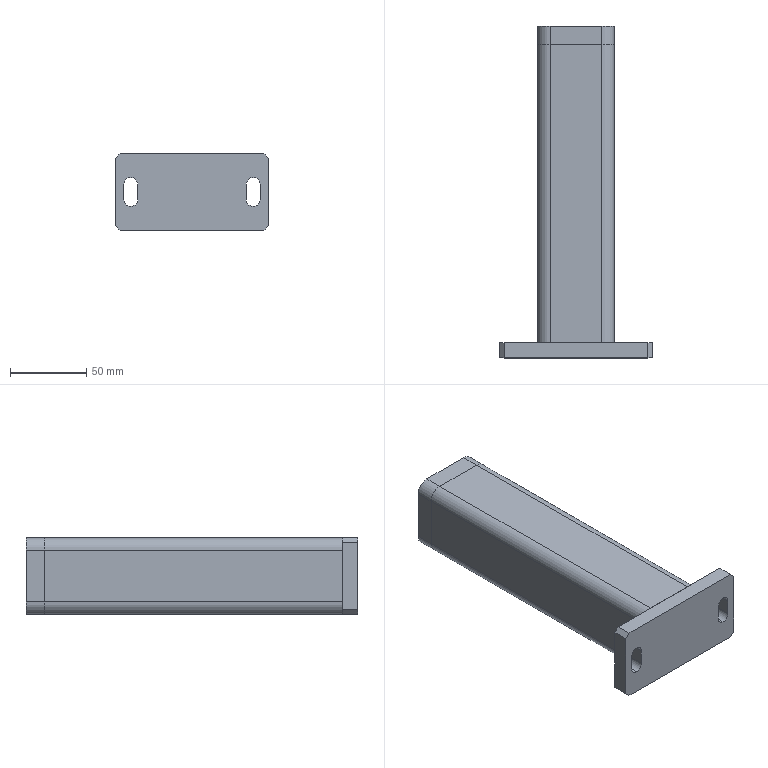Part | SolidWorks | features BaseBody 3 | 3 solids | 50 faces | box 100 x 217 x 50 mm | volume 210593 mm3 | plane 30 | cylinder 20 | commonest cylinder face diameters 16 x8 9 x6 8 x4 10.2 x2
STEP:
#1=CARTESIAN_POINT('',(21.,0.,-17.));
#2=VERTEX_POINT('',#1);
#3=CARTESIAN_POINT('',(17.,0.,-21.));
#4=VERTEX_POINT('',#3);
#5=CARTESIAN_POINT('',(17.,0.,-17.));
#6=DIRECTION('',(0.,1.,0.));
#7=DIRECTION('',(0.,0.,1.));
#8=AXIS2_PLACEMENT_3D('',#5,#6,#7);
#9=CIRCLE('',#8,4.);
#10=EDGE_CURVE('',#2,#4,#9,.T.);
#11=ORIENTED_EDGE('',*,*,#10,.T.);
#12=CARTESIAN_POINT('',(-17.,0.,-21.));
#13=VERTEX_POINT('',#12);
#14=CARTESIAN_POINT('',(-17.,0.,-21.));
#15=DIRECTION('',(-1.,0.,0.));
#16=VECTOR('',#15,1000.);
#17=LINE('',#14,#16);
#18=EDGE_CURVE('',#4,#13,#17,.T.);
#19=ORIENTED_EDGE('',*,*,#18,.T.);
#20=CARTESIAN_POINT('',(-21.,0.,-17.));
#21=VERTEX_POINT('',#20);
#22=CARTESIAN_POINT('',(-17.,0.,-17.));
#23=DIRECTION('',(0.,1.,0.));
#24=DIRECTION('',(0.,0.,1.));
#25=AXIS2_PLACEMENT_3D('',#22,#23,#24);
#26=CIRCLE('',#25,4.);
#27=EDGE_CURVE('',#13,#21,#26,.T.);
#28=ORIENTED_EDGE('',*,*,#27,.T.);
#29=CARTESIAN_POINT('',(-21.,0.,17.));
#30=VERTEX_POINT('',#29);
#31=CARTESIAN_POINT('',(-21.,0.,-17.));
#32=DIRECTION('',(0.,0.,1.));
#33=VECTOR('',#32,1000.);
#34=LINE('',#31,#33);
#35=EDGE_CURVE('',#21,#30,#34,.T.);
#36=ORIENTED_EDGE('',*,*,#35,.T.);
#37=CARTESIAN_POINT('',(-17.,0.,21.));
#38=VERTEX_POINT('',#37);
#39=CARTESIAN_POINT('',(-17.,0.,17.));
#40=DIRECTION('',(0.,1.,0.));
#41=DIRECTION('',(0.,0.,1.));
#42=AXIS2_PLACEMENT_3D('',#39,#40,#41);
#43=CIRCLE('',#42,4.);
#44=EDGE_CURVE('',#30,#38,#43,.T.);
#45=ORIENTED_EDGE('',*,*,#44,.T.);
#46=CARTESIAN_POINT('',(17.,0.,21.));
#47=VERTEX_POINT('',#46);
#48=CARTESIAN_POINT('',(17.,0.,21.));
#49=DIRECTION('',(1.,0.,0.));
#50=VECTOR('',#49,1000.);
#51=LINE('',#48,#50);
#52=EDGE_CURVE('',#38,#47,#51,.T.);
#53=ORIENTED_EDGE('',*,*,#52,.T.);
#54=CARTESIAN_POINT('',(21.,0.,17.));
#55=VERTEX_POINT('',#54);
#56=CARTESIAN_POINT('',(17.,0.,17.));
#57=DIRECTION('',(0.,1.,0.));
#58=DIRECTION('',(0.,0.,1.));
#59=AXIS2_PLACEMENT_3D('',#56,#57,#58);
#60=CIRCLE('',#59,4.);
#61=EDGE_CURVE('',#47,#55,#60,.T.);
#62=ORIENTED_EDGE('',*,*,#61,.T.);
#63=CARTESIAN_POINT('',(21.,0.,17.));
#64=DIRECTION('',(0.,0.,-1.));
#65=VECTOR('',#64,1000.);
#66=LINE('',#63,#65);
#67=EDGE_CURVE('',#55,#2,#66,.T.);
#68=ORIENTED_EDGE('',*,*,#67,.T.);
#69=EDGE_LOOP('',(#11,#19,#28,#36,#45,#53,#62,#68));
#70=FACE_BOUND('',#69,.T.);
#71=CARTESIAN_POINT('',(17.,0.,25.));
#72=VERTEX_POINT('',#71);
#73=CARTESIAN_POINT('',(25.,0.,17.));
#74=VERTEX_POINT('',#73);
#75=CARTESIAN_POINT('',(17.,0.,17.));
#76=DIRECTION('',(0.,1.,0.));
#77=DIRECTION('',(0.,0.,1.));
#78=AXIS2_PLACEMENT_3D('',#75,#76,#77);
#79=CIRCLE('',#78,8.);
#80=EDGE_CURVE('',#72,#74,#79,.T.);
#81=ORIENTED_EDGE('',*,*,#80,.F.);
#82=CARTESIAN_POINT('',(-17.,0.,25.));
#83=VERTEX_POINT('',#82);
#84=CARTESIAN_POINT('',(17.,0.,25.));
#85=DIRECTION('',(1.,0.,0.));
#86=VECTOR('',#85,1000.);
#87=LINE('',#84,#86);
#88=EDGE_CURVE('',#83,#72,#87,.T.);
#89=ORIENTED_EDGE('',*,*,#88,.F.);
#90=CARTESIAN_POINT('',(-25.,0.,17.));
#91=VERTEX_POINT('',#90);
#92=CARTESIAN_POINT('',(-17.,0.,17.));
#93=DIRECTION('',(0.,1.,0.));
#94=DIRECTION('',(0.,0.,1.));
#95=AXIS2_PLACEMENT_3D('',#92,#93,#94);
#96=CIRCLE('',#95,8.);
#97=EDGE_CURVE('',#91,#83,#96,.T.);
#98=ORIENTED_EDGE('',*,*,#97,.F.);
#99=CARTESIAN_POINT('',(-25.,0.,-17.));
#100=VERTEX_POINT('',#99);
#101=CARTESIAN_POINT('',(-25.,0.,-17.));
#102=DIRECTION('',(0.,0.,1.));
#103=VECTOR('',#102,1000.);
#104=LINE('',#101,#103);
#105=EDGE_CURVE('',#100,#91,#104,.T.);
#106=ORIENTED_EDGE('',*,*,#105,.F.);
#107=CARTESIAN_POINT('',(-17.,0.,-25.));
#108=VERTEX_POINT('',#107);
#109=CARTESIAN_POINT('',(-17.,0.,-17.));
#110=DIRECTION('',(0.,1.,0.));
#111=DIRECTION('',(0.,0.,1.));
#112=AXIS2_PLACEMENT_3D('',#109,#110,#111);
#113=CIRCLE('',#112,8.);
#114=EDGE_CURVE('',#108,#100,#113,.T.);
#115=ORIENTED_EDGE('',*,*,#114,.F.);
#116=CARTESIAN_POINT('',(17.,0.,-25.));
#117=VERTEX_POINT('',#116);
#118=CARTESIAN_POINT('',(-17.,0.,-25.));
#119=DIRECTION('',(-1.,0.,0.));
#120=VECTOR('',#119,1000.);
#121=LINE('',#118,#120);
#122=EDGE_CURVE('',#117,#108,#121,.T.);
#123=ORIENTED_EDGE('',*,*,#122,.F.);
#124=CARTESIAN_POINT('',(25.,0.,-17.));
#125=VERTEX_POINT('',#124);
#126=CARTESIAN_POINT('',(17.,0.,-17.));
#127=DIRECTION('',(0.,1.,0.));
#128=DIRECTION('',(0.,0.,1.));
#129=AXIS2_PLACEMENT_3D('',#126,#127,#128);
#130=CIRCLE('',#129,8.);
#131=EDGE_CURVE('',#125,#117,#130,.T.);
#132=ORIENTED_EDGE('',*,*,#131,.F.);
#133=CARTESIAN_POINT('',(25.,0.,17.));
#134=DIRECTION('',(0.,0.,-1.));
#135=VECTOR('',#134,1000.);
#136=LINE('',#133,#135);
#137=EDGE_CURVE('',#74,#125,#136,.T.);
#138=ORIENTED_EDGE('',*,*,#137,.F.);
#139=EDGE_LOOP('',(#81,#89,#98,#106,#115,#123,#132,#138));
#140=FACE_OUTER_BOUND('',#139,.T.);
#141=CARTESIAN_POINT('',(17.,0.,17.));
#142=DIRECTION('',(0.,1.,0.));
#143=DIRECTION('',(1.,0.,0.));
#144=AXIS2_PLACEMENT_3D('',#141,#142,#143);
#145=PLANE('',#144);
#146=ADVANCED_FACE('',(#70,#140),#145,.F.);
#147=CARTESIAN_POINT('',(21.,195.,-17.));
#148=VERTEX_POINT('',#147);
#149=CARTESIAN_POINT('',(17.,195.,-21.));
#150=VERTEX_POINT('',#149);
#151=CARTESIAN_POINT('',(17.,195.,-17.));
#152=DIRECTION('',(0.,1.,0.));
#153=DIRECTION('',(0.,0.,1.));
#154=AXIS2_PLACEMENT_3D('',#151,#152,#153);
#155=CIRCLE('',#154,4.);
#156=EDGE_CURVE('',#148,#150,#155,.T.);
#157=ORIENTED_EDGE('',*,*,#156,.F.);
#158=CARTESIAN_POINT('',(21.,195.,17.));
#159=VERTEX_POINT('',#158);
#160=CARTESIAN_POINT('',(21.,195.,17.));
#161=DIRECTION('',(0.,0.,-1.));
#162=VECTOR('',#161,1000.);
#163=LINE('',#160,#162);
#164=EDGE_CURVE('',#159,#148,#163,.T.);
#165=ORIENTED_EDGE('',*,*,#164,.F.);
#166=CARTESIAN_POINT('',(17.,195.,21.));
#167=VERTEX_POINT('',#166);
#168=CARTESIAN_POINT('',(17.,195.,17.));
#169=DIRECTION('',(0.,1.,0.));
#170=DIRECTION('',(0.,0.,1.));
#171=AXIS2_PLACEMENT_3D('',#168,#169,#170);
#172=CIRCLE('',#171,4.);
#173=EDGE_CURVE('',#167,#159,#172,.T.);
#174=ORIENTED_EDGE('',*,*,#173,.F.);
#175=CARTESIAN_POINT('',(-17.,195.,21.));
#176=VERTEX_POINT('',#175);
#177=CARTESIAN_POINT('',(17.,195.,21.));
#178=DIRECTION('',(1.,0.,0.));
#179=VECTOR('',#178,1000.);
#180=LINE('',#177,#179);
#181=EDGE_CURVE('',#176,#167,#180,.T.);
#182=ORIENTED_EDGE('',*,*,#181,.F.);
#183=CARTESIAN_POINT('',(-21.,195.,17.));
#184=VERTEX_POINT('',#183);
#185=CARTESIAN_POINT('',(-17.,195.,17.));
#186=DIRECTION('',(0.,1.,0.));
#187=DIRECTION('',(0.,0.,1.));
#188=AXIS2_PLACEMENT_3D('',#185,#186,#187);
#189=CIRCLE('',#188,4.);
#190=EDGE_CURVE('',#184,#176,#189,.T.);
#191=ORIENTED_EDGE('',*,*,#190,.F.);
#192=CARTESIAN_POINT('',(-21.,195.,-17.));
#193=VERTEX_POINT('',#192);
#194=CARTESIAN_POINT('',(-21.,195.,-17.));
#195=DIRECTION('',(0.,0.,1.));
#196=VECTOR('',#195,1000.);
#197=LINE('',#194,#196);
#198=EDGE_CURVE('',#193,#184,#197,.T.);
#199=ORIENTED_EDGE('',*,*,#198,.F.);
#200=CARTESIAN_POINT('',(-17.,195.,-21.));
#201=VERTEX_POINT('',#200);
#202=CARTESIAN_POINT('',(-17.,195.,-17.));
#203=DIRECTION('',(0.,1.,0.));
#204=DIRECTION('',(0.,0.,1.));
#205=AXIS2_PLACEMENT_3D('',#202,#203,#204);
#206=CIRCLE('',#205,4.);
#207=EDGE_CURVE('',#201,#193,#206,.T.);
#208=ORIENTED_EDGE('',*,*,#207,.F.);
#209=CARTESIAN_POINT('',(-17.,195.,-21.));
#210=DIRECTION('',(-1.,0.,0.));
#211=VECTOR('',#210,1000.);
#212=LINE('',#209,#211);
#213=EDGE_CURVE('',#150,#201,#212,.T.);
#214=ORIENTED_EDGE('',*,*,#213,.F.);
#215=EDGE_LOOP('',(#157,#165,#174,#182,#191,#199,#208,#214));
#216=FACE_BOUND('',#215,.T.);
#217=CARTESIAN_POINT('',(17.,195.,25.));
#218=VERTEX_POINT('',#217);
#219=CARTESIAN_POINT('',(25.,195.,17.));
#220=VERTEX_POINT('',#219);
#221=CARTESIAN_POINT('',(17.,195.,17.));
#222=DIRECTION('',(0.,1.,0.));
#223=DIRECTION('',(0.,0.,1.));
#224=AXIS2_PLACEMENT_3D('',#221,#222,#223);
#225=CIRCLE('',#224,8.);
#226=EDGE_CURVE('',#218,#220,#225,.T.);
#227=ORIENTED_EDGE('',*,*,#226,.T.);
#228=CARTESIAN_POINT('',(25.,195.,-17.));
#229=VERTEX_POINT('',#228);
#230=CARTESIAN_POINT('',(25.,195.,17.));
#231=DIRECTION('',(0.,0.,-1.));
#232=VECTOR('',#231,1000.);
#233=LINE('',#230,#232);
#234=EDGE_CURVE('',#220,#229,#233,.T.);
#235=ORIENTED_EDGE('',*,*,#234,.T.);
#236=CARTESIAN_POINT('',(17.,195.,-25.));
#237=VERTEX_POINT('',#236);
#238=CARTESIAN_POINT('',(17.,195.,-17.));
#239=DIRECTION('',(0.,1.,0.));
#240=DIRECTION('',(0.,0.,1.));
#241=AXIS2_PLACEMENT_3D('',#238,#239,#240);
#242=CIRCLE('',#241,8.);
#243=EDGE_CURVE('',#229,#237,#242,.T.);
#244=ORIENTED_EDGE('',*,*,#243,.T.);
#245=CARTESIAN_POINT('',(-17.,195.,-25.));
#246=VERTEX_POINT('',#245);
#247=CARTESIAN_POINT('',(-17.,195.,-25.));
#248=DIRECTION('',(-1.,0.,0.));
#249=VECTOR('',#248,1000.);
#250=LINE('',#247,#249);
#251=EDGE_CURVE('',#237,#246,#250,.T.);
#252=ORIENTED_EDGE('',*,*,#251,.T.);
#253=CARTESIAN_POINT('',(-25.,195.,-17.));
#254=VERTEX_POINT('',#253);
#255=CARTESIAN_POINT('',(-17.,195.,-17.));
#256=DIRECTION('',(0.,1.,0.));
#257=DIRECTION('',(0.,0.,1.));
#258=AXIS2_PLACEMENT_3D('',#255,#256,#257);
#259=CIRCLE('',#258,8.);
#260=EDGE_CURVE('',#246,#254,#259,.T.);
#261=ORIENTED_EDGE('',*,*,#260,.T.);
#262=CARTESIAN_POINT('',(-25.,195.,17.));
#263=VERTEX_POINT('',#262);
#264=CARTESIAN_POINT('',(-25.,195.,-17.));
#265=DIRECTION('',(0.,0.,1.));
#266=VECTOR('',#265,1000.);
#267=LINE('',#264,#266);
#268=EDGE_CURVE('',#254,#263,#267,.T.);
#269=ORIENTED_EDGE('',*,*,#268,.T.);
#270=CARTESIAN_POINT('',(-17.,195.,25.));
#271=VERTEX_POINT('',#270);
#272=CARTESIAN_POINT('',(-17.,195.,17.));
#273=DIRECTION('',(0.,1.,0.));
#274=DIRECTION('',(0.,0.,1.));
#275=AXIS2_PLACEMENT_3D('',#272,#273,#274);
#276=CIRCLE('',#275,8.);
#277=EDGE_CURVE('',#263,#271,#276,.T.);
#278=ORIENTED_EDGE('',*,*,#277,.T.);
#279=CARTESIAN_POINT('',(17.,195.,25.));
#280=DIRECTION('',(1.,0.,0.));
#281=VECTOR('',#280,1000.);
#282=LINE('',#279,#281);
#283=EDGE_CURVE('',#271,#218,#282,.T.);
#284=ORIENTED_EDGE('',*,*,#283,.T.);
#285=EDGE_LOOP('',(#227,#235,#244,#252,#261,#269,#278,#284));
#286=FACE_OUTER_BOUND('',#285,.T.);
#287=CARTESIAN_POINT('',(17.,195.,17.));
#288=DIRECTION('',(0.,1.,0.));
#289=DIRECTION('',(1.,0.,0.));
#290=AXIS2_PLACEMENT_3D('',#287,#288,#289);
#291=PLANE('',#290);
#292=ADVANCED_FACE('',(#216,#286),#291,.T.);
#293=ORIENTED_EDGE('',*,*,#88,.T.);
#294=CARTESIAN_POINT('',(17.,195.,25.));
#295=DIRECTION('',(0.,-1.,0.));
#296=VECTOR('',#295,1000.);
#297=LINE('',#294,#296);
#298=EDGE_CURVE('',#218,#72,#297,.T.);
#299=ORIENTED_EDGE('',*,*,#298,.F.);
#300=ORIENTED_EDGE('',*,*,#283,.F.);
#301=CARTESIAN_POINT('',(-17.,195.,25.));
#302=DIRECTION('',(0.,-1.,0.));
#303=VECTOR('',#302,1000.);
#304=LINE('',#301,#303);
#305=EDGE_CURVE('',#271,#83,#304,.T.);
#306=ORIENTED_EDGE('',*,*,#305,.T.);
#307=EDGE_LOOP('',(#293,#299,#300,#306));
#308=FACE_OUTER_BOUND('',#307,.T.);
#309=CARTESIAN_POINT('',(17.,195.,25.));
#310=DIRECTION('',(0.,0.,-1.));
#311=DIRECTION('',(0.,-1.,0.));
#312=AXIS2_PLACEMENT_3D('',#309,#310,#311);
#313=PLANE('',#312);
#314=ADVANCED_FACE('',(#308),#313,.F.);
#315=ORIENTED_EDGE('',*,*,#18,.F.);
#316=CARTESIAN_POINT('',(17.,195.,-21.));
#317=DIRECTION('',(0.,-1.,0.));
#318=VECTOR('',#317,1000.);
#319=LINE('',#316,#318);
#320=EDGE_CURVE('',#150,#4,#319,.T.);
#321=ORIENTED_EDGE('',*,*,#320,.F.);
#322=ORIENTED_EDGE('',*,*,#213,.T.);
#323=CARTESIAN_POINT('',(-17.,195.,-21.));
#324=DIRECTION('',(0.,-1.,0.));
#325=VECTOR('',#324,1000.);
#326=LINE('',#323,#325);
#327=EDGE_CURVE('',#201,#13,#326,.T.);
#328=ORIENTED_EDGE('',*,*,#327,.T.);
#329=EDGE_LOOP('',(#315,#321,#322,#328));
#330=FACE_OUTER_BOUND('',#329,.T.);
#331=CARTESIAN_POINT('',(-17.,195.,-21.));
#332=DIRECTION('',(0.,0.,1.));
#333=DIRECTION('',(1.,0.,0.));
#334=AXIS2_PLACEMENT_3D('',#331,#332,#333);
#335=PLANE('',#334);
#336=ADVANCED_FACE('',(#330),#335,.T.);
#337=ORIENTED_EDGE('',*,*,#27,.F.);
#338=ORIENTED_EDGE('',*,*,#327,.F.);
#339=ORIENTED_EDGE('',*,*,#207,.T.);
#340=CARTESIAN_POINT('',(-21.,195.,-17.));
#341=DIRECTION('',(0.,-1.,0.));
#342=VECTOR('',#341,1000.);
#343=LINE('',#340,#342);
#344=EDGE_CURVE('',#193,#21,#343,.T.);
#345=ORIENTED_EDGE('',*,*,#344,.T.);
#346=EDGE_LOOP('',(#337,#338,#339,#345));
#347=FACE_OUTER_BOUND('',#346,.T.);
#348=CARTESIAN_POINT('',(-17.,195.,-17.));
#349=DIRECTION('',(0.,-1.,0.));
#350=DIRECTION('',(0.,0.,-1.));
#351=AXIS2_PLACEMENT_3D('',#348,#349,#350);
#352=CYLINDRICAL_SURFACE('',#351,4.);
#353=ADVANCED_FACE('',(#347),#352,.F.);
#354=ORIENTED_EDGE('',*,*,#35,.F.);
#355=ORIENTED_EDGE('',*,*,#344,.F.);
#356=ORIENTED_EDGE('',*,*,#198,.T.);
#357=CARTESIAN_POINT('',(-21.,195.,17.));
#358=DIRECTION('',(0.,-1.,0.));
#359=VECTOR('',#358,1000.);
#360=LINE('',#357,#359);
#361=EDGE_CURVE('',#184,#30,#360,.T.);
#362=ORIENTED_EDGE('',*,*,#361,.T.);
#363=EDGE_LOOP('',(#354,#355,#356,#362));
#364=FACE_OUTER_BOUND('',#363,.T.);
#365=CARTESIAN_POINT('',(-21.,195.,-17.));
#366=DIRECTION('',(1.,0.,0.));
#367=DIRECTION('',(0.,1.,0.));
#368=AXIS2_PLACEMENT_3D('',#365,#366,#367);
#369=PLANE('',#368);
#370=ADVANCED_FACE('',(#364),#369,.T.);
#371=ORIENTED_EDGE('',*,*,#44,.F.);
#372=ORIENTED_EDGE('',*,*,#361,.F.);
#373=ORIENTED_EDGE('',*,*,#190,.T.);
#374=CARTESIAN_POINT('',(-17.,195.,21.));
#375=DIRECTION('',(0.,-1.,0.));
#376=VECTOR('',#375,1000.);
#377=LINE('',#374,#376);
#378=EDGE_CURVE('',#176,#38,#377,.T.);
#379=ORIENTED_EDGE('',*,*,#378,.T.);
#380=EDGE_LOOP('',(#371,#372,#373,#379));
#381=FACE_OUTER_BOUND('',#380,.T.);
#382=CARTESIAN_POINT('',(-17.,195.,17.));
#383=DIRECTION('',(0.,-1.,0.));
#384=DIRECTION('',(0.,0.,-1.));
#385=AXIS2_PLACEMENT_3D('',#382,#383,#384);
#386=CYLINDRICAL_SURFACE('',#385,4.);
#387=ADVANCED_FACE('',(#381),#386,.F.);
#388=ORIENTED_EDGE('',*,*,#52,.F.);
#389=ORIENTED_EDGE('',*,*,#378,.F.);
#390=ORIENTED_EDGE('',*,*,#181,.T.);
#391=CARTESIAN_POINT('',(17.,195.,21.));
#392=DIRECTION('',(0.,-1.,0.));
#393=VECTOR('',#392,1000.);
#394=LINE('',#391,#393);
#395=EDGE_CURVE('',#167,#47,#394,.T.);
#396=ORIENTED_EDGE('',*,*,#395,.T.);
#397=EDGE_LOOP('',(#388,#389,#390,#396));
#398=FACE_OUTER_BOUND('',#397,.T.);
#399=CARTESIAN_POINT('',(17.,195.,21.));
#400=DIRECTION('',(0.,0.,-1.));
#401=DIRECTION('',(0.,-1.,0.));
#402=AXIS2_PLACEMENT_3D('',#399,#400,#401);
#403=PLANE('',#402);
#404=ADVANCED_FACE('',(#398),#403,.T.);
#405=ORIENTED_EDGE('',*,*,#61,.F.);
#406=ORIENTED_EDGE('',*,*,#395,.F.);
#407=ORIENTED_EDGE('',*,*,#173,.T.);
#408=CARTESIAN_POINT('',(21.,195.,17.));
#409=DIRECTION('',(0.,-1.,0.));
#410=VECTOR('',#409,1000.);
#411=LINE('',#408,#410);
#412=EDGE_CURVE('',#159,#55,#411,.T.);
#413=ORIENTED_EDGE('',*,*,#412,.T.);
#414=EDGE_LOOP('',(#405,#406,#407,#413));
#415=FACE_OUTER_BOUND('',#414,.T.);
#416=CARTESIAN_POINT('',(17.,195.,17.));
#417=DIRECTION('',(0.,-1.,0.));
#418=DIRECTION('',(0.,0.,-1.));
#419=AXIS2_PLACEMENT_3D('',#416,#417,#418);
#420=CYLINDRICAL_SURFACE('',#419,4.);
#421=ADVANCED_FACE('',(#415),#420,.F.);
#422=ORIENTED_EDGE('',*,*,#67,.F.);
#423=ORIENTED_EDGE('',*,*,#412,.F.);
#424=ORIENTED_EDGE('',*,*,#164,.T.);
#425=CARTESIAN_POINT('',(21.,195.,-17.));
#426=DIRECTION('',(0.,-1.,0.));
#427=VECTOR('',#426,1000.);
#428=LINE('',#425,#427);
#429=EDGE_CURVE('',#148,#2,#428,.T.);
#430=ORIENTED_EDGE('',*,*,#429,.T.);
#431=EDGE_LOOP('',(#422,#423,#424,#430));
#432=FACE_OUTER_BOUND('',#431,.T.);
#433=CARTESIAN_POINT('',(21.,195.,17.));
#434=DIRECTION('',(-1.,0.,0.));
#435=DIRECTION('',(0.,0.,1.));
#436=AXIS2_PLACEMENT_3D('',#433,#434,#435);
#437=PLANE('',#436);
#438=ADVANCED_FACE('',(#432),#437,.T.);
#439=ORIENTED_EDGE('',*,*,#10,.F.);
#440=ORIENTED_EDGE('',*,*,#429,.F.);
#441=ORIENTED_EDGE('',*,*,#156,.T.);
#442=ORIENTED_EDGE('',*,*,#320,.T.);
#443=EDGE_LOOP('',(#439,#440,#441,#442));
#444=FACE_OUTER_BOUND('',#443,.T.);
#445=CARTESIAN_POINT('',(17.,195.,-17.));
#446=DIRECTION('',(0.,-1.,0.));
#447=DIRECTION('',(0.,0.,-1.));
#448=AXIS2_PLACEMENT_3D('',#445,#446,#447);
#449=CYLINDRICAL_SURFACE('',#448,4.);
#450=ADVANCED_FACE('',(#444),#449,.F.);
#451=ORIENTED_EDGE('',*,*,#97,.T.);
#452=ORIENTED_EDGE('',*,*,#305,.F.);
#453=ORIENTED_EDGE('',*,*,#277,.F.);
#454=CARTESIAN_POINT('',(-25.,195.,17.));
#455=DIRECTION('',(0.,-1.,0.));
#456=VECTOR('',#455,1000.);
#457=LINE('',#454,#456);
#458=EDGE_CURVE('',#263,#91,#457,.T.);
#459=ORIENTED_EDGE('',*,*,#458,.T.);
#460=EDGE_LOOP('',(#451,#452,#453,#459));
#461=FACE_OUTER_BOUND('',#460,.T.);
#462=CARTESIAN_POINT('',(-17.,195.,17.));
#463=DIRECTION('',(0.,-1.,0.));
#464=DIRECTION('',(0.,0.,-1.));
#465=AXIS2_PLACEMENT_3D('',#462,#463,#464);
#466=CYLINDRICAL_SURFACE('',#465,8.);
#467=ADVANCED_FACE('',(#461),#466,.T.);
#468=ORIENTED_EDGE('',*,*,#105,.T.);
#469=ORIENTED_EDGE('',*,*,#458,.F.);
#470=ORIENTED_EDGE('',*,*,#268,.F.);
#471=CARTESIAN_POINT('',(-25.,195.,-17.));
#472=DIRECTION('',(0.,-1.,0.));
#473=VECTOR('',#472,1000.);
#474=LINE('',#471,#473);
#475=EDGE_CURVE('',#254,#100,#474,.T.);
#476=ORIENTED_EDGE('',*,*,#475,.T.);
#477=EDGE_LOOP('',(#468,#469,#470,#476));
#478=FACE_OUTER_BOUND('',#477,.T.);
#479=CARTESIAN_POINT('',(-25.,195.,-17.));
#480=DIRECTION('',(1.,0.,0.));
#481=DIRECTION('',(0.,1.,0.));
#482=AXIS2_PLACEMENT_3D('',#479,#480,#481);
#483=PLANE('',#482);
#484=ADVANCED_FACE('',(#478),#483,.F.);
#485=ORIENTED_EDGE('',*,*,#114,.T.);
#486=ORIENTED_EDGE('',*,*,#475,.F.);
#487=ORIENTED_EDGE('',*,*,#260,.F.);
#488=CARTESIAN_POINT('',(-17.,195.,-25.));
#489=DIRECTION('',(0.,-1.,0.));
#490=VECTOR('',#489,1000.);
#491=LINE('',#488,#490);
#492=EDGE_CURVE('',#246,#108,#491,.T.);
#493=ORIENTED_EDGE('',*,*,#492,.T.);
#494=EDGE_LOOP('',(#485,#486,#487,#493));
#495=FACE_OUTER_BOUND('',#494,.T.);
#496=CARTESIAN_POINT('',(-17.,195.,-17.));
#497=DIRECTION('',(0.,-1.,0.));
#498=DIRECTION('',(0.,0.,-1.));
#499=AXIS2_PLACEMENT_3D('',#496,#497,#498);
#500=CYLINDRICAL_SURFACE('',#499,8.);
#501=ADVANCED_FACE('',(#495),#500,.T.);
#502=ORIENTED_EDGE('',*,*,#122,.T.);
#503=ORIENTED_EDGE('',*,*,#492,.F.);
#504=ORIENTED_EDGE('',*,*,#251,.F.);
#505=CARTESIAN_POINT('',(17.,195.,-25.));
#506=DIRECTION('',(0.,-1.,0.));
#507=VECTOR('',#506,1000.);
#508=LINE('',#505,#507);
#509=EDGE_CURVE('',#237,#117,#508,.T.);
#510=ORIENTED_EDGE('',*,*,#509,.T.);
#511=EDGE_LOOP('',(#502,#503,#504,#510));
#512=FACE_OUTER_BOUND('',#511,.T.);
#513=CARTESIAN_POINT('',(-17.,195.,-25.));
#514=DIRECTION('',(0.,0.,1.));
#515=DIRECTION('',(1.,0.,0.));
#516=AXIS2_PLACEMENT_3D('',#513,#514,#515);
#517=PLANE('',#516);
#518=ADVANCED_FACE('',(#512),#517,.F.);
#519=ORIENTED_EDGE('',*,*,#131,.T.);
#520=ORIENTED_EDGE('',*,*,#509,.F.);
#521=ORIENTED_EDGE('',*,*,#243,.F.);
#522=CARTESIAN_POINT('',(25.,195.,-17.));
#523=DIRECTION('',(0.,-1.,0.));
#524=VECTOR('',#523,1000.);
#525=LINE('',#522,#524);
#526=EDGE_CURVE('',#229,#125,#525,.T.);
#527=ORIENTED_EDGE('',*,*,#526,.T.);
#528=EDGE_LOOP('',(#519,#520,#521,#527));
#529=FACE_OUTER_BOUND('',#528,.T.);
#530=CARTESIAN_POINT('',(17.,195.,-17.));
#531=DIRECTION('',(0.,-1.,0.));
#532=DIRECTION('',(0.,0.,-1.));
#533=AXIS2_PLACEMENT_3D('',#530,#531,#532);
#534=CYLINDRICAL_SURFACE('',#533,8.);
#535=ADVANCED_FACE('',(#529),#534,.T.);
#536=ORIENTED_EDGE('',*,*,#137,.T.);
#537=ORIENTED_EDGE('',*,*,#526,.F.);
#538=ORIENTED_EDGE('',*,*,#234,.F.);
#539=CARTESIAN_POINT('',(25.,195.,17.));
#540=DIRECTION('',(0.,-1.,0.));
#541=VECTOR('',#540,1000.);
#542=LINE('',#539,#541);
#543=EDGE_CURVE('',#220,#74,#542,.T.);
#544=ORIENTED_EDGE('',*,*,#543,.T.);
#545=EDGE_LOOP('',(#536,#537,#538,#544));
#546=FACE_OUTER_BOUND('',#545,.T.);
#547=CARTESIAN_POINT('',(25.,195.,17.));
#548=DIRECTION('',(-1.,0.,0.));
#549=DIRECTION('',(0.,0.,1.));
#550=AXIS2_PLACEMENT_3D('',#547,#548,#549);
#551=PLANE('',#550);
#552=ADVANCED_FACE('',(#546),#551,.F.);
#553=ORIENTED_EDGE('',*,*,#80,.T.);
#554=ORIENTED_EDGE('',*,*,#543,.F.);
#555=ORIENTED_EDGE('',*,*,#226,.F.);
#556=ORIENTED_EDGE('',*,*,#298,.T.);
#557=EDGE_LOOP('',(#553,#554,#555,#556));
#558=FACE_OUTER_BOUND('',#557,.T.);
#559=CARTESIAN_POINT('',(17.,195.,17.));
#560=DIRECTION('',(0.,-1.,0.));
#561=DIRECTION('',(0.,0.,-1.));
#562=AXIS2_PLACEMENT_3D('',#559,#560,#561);
#563=CYLINDRICAL_SURFACE('',#562,8.);
#564=ADVANCED_FACE('',(#558),#563,.T.);
#565=CLOSED_SHELL('',(#146,#292,#314,#336,#353,#370,#387,#404,#421,#438,#450,#467,#484,#501,#518,#535,#552,#564));
#566=MANIFOLD_SOLID_BREP('',#565);
#567=CARTESIAN_POINT('',(0.,195.,-5.1));
#568=VERTEX_POINT('',#567);
#569=CARTESIAN_POINT('',(0.,207.,-5.1));
#570=VERTEX_POINT('',#569);
#571=CARTESIAN_POINT('',(0.,207.,-5.1));
#572=DIRECTION('',(0.,1.,0.));
#573=VECTOR('',#572,1000.);
#574=LINE('',#571,#573);
#575=EDGE_CURVE('',#568,#570,#574,.T.);
#576=ORIENTED_EDGE('',*,*,#575,.F.);
#577=CARTESIAN_POINT('',(0.,195.,5.1));
#578=VERTEX_POINT('',#577);
#579=CARTESIAN_POINT('',(0.,195.,0.));
#580=DIRECTION('',(0.,1.,0.));
#581=DIRECTION('',(0.,0.,1.));
#582=AXIS2_PLACEMENT_3D('',#579,#580,#581);
#583=CIRCLE('',#582,5.1);
#584=EDGE_CURVE('',#578,#568,#583,.T.);
#585=ORIENTED_EDGE('',*,*,#584,.F.);
#586=CARTESIAN_POINT('',(0.,207.,5.1));
#587=VERTEX_POINT('',#586);
#588=CARTESIAN_POINT('',(0.,207.,5.1));
#589=DIRECTION('',(0.,1.,0.));
#590=VECTOR('',#589,1000.);
#591=LINE('',#588,#590);
#592=EDGE_CURVE('',#578,#587,#591,.T.);
#593=ORIENTED_EDGE('',*,*,#592,.T.);
#594=CARTESIAN_POINT('',(0.,207.,0.));
#595=DIRECTION('',(0.,1.,0.));
#596=DIRECTION('',(0.,0.,1.));
#597=AXIS2_PLACEMENT_3D('',#594,#595,#596);
#598=CIRCLE('',#597,5.1);
#599=EDGE_CURVE('',#587,#570,#598,.T.);
#600=ORIENTED_EDGE('',*,*,#599,.T.);
#601=EDGE_LOOP('',(#576,#585,#593,#600));
#602=FACE_OUTER_BOUND('',#601,.T.);
#603=CARTESIAN_POINT('',(0.,207.,0.));
#604=DIRECTION('',(0.,1.,0.));
#605=DIRECTION('',(0.,0.,1.));
#606=AXIS2_PLACEMENT_3D('',#603,#604,#605);
#607=CYLINDRICAL_SURFACE('',#606,5.1);
#608=ADVANCED_FACE('',(#602),#607,.F.);
#609=ORIENTED_EDGE('',*,*,#584,.T.);
#610=CARTESIAN_POINT('',(0.,195.,0.));
#611=DIRECTION('',(0.,1.,0.));
#612=DIRECTION('',(0.,0.,1.));
#613=AXIS2_PLACEMENT_3D('',#610,#611,#612);
#614=CIRCLE('',#613,5.1);
#615=EDGE_CURVE('',#568,#578,#614,.T.);
#616=ORIENTED_EDGE('',*,*,#615,.T.);
#617=EDGE_LOOP('',(#609,#616));
#618=FACE_BOUND('',#617,.T.);
#619=CARTESIAN_POINT('',(17.,195.,25.));
#620=VERTEX_POINT('',#619);
#621=CARTESIAN_POINT('',(25.,195.,17.));
#622=VERTEX_POINT('',#621);
#623=CARTESIAN_POINT('',(17.,195.,17.));
#624=DIRECTION('',(0.,1.,0.));
#625=DIRECTION('',(0.,0.,1.));
#626=AXIS2_PLACEMENT_3D('',#623,#624,#625);
#627=CIRCLE('',#626,8.);
#628=EDGE_CURVE('',#620,#622,#627,.T.);
#629=ORIENTED_EDGE('',*,*,#628,.F.);
#630=CARTESIAN_POINT('',(-17.,195.,25.));
#631=VERTEX_POINT('',#630);
#632=CARTESIAN_POINT('',(-17.,195.,25.));
#633=DIRECTION('',(1.,0.,0.));
#634=VECTOR('',#633,1000.);
#635=LINE('',#632,#634);
#636=EDGE_CURVE('',#631,#620,#635,.T.);
#637=ORIENTED_EDGE('',*,*,#636,.F.);
#638=CARTESIAN_POINT('',(-25.,195.,17.));
#639=VERTEX_POINT('',#638);
#640=CARTESIAN_POINT('',(-17.,195.,17.));
#641=DIRECTION('',(0.,1.,0.));
#642=DIRECTION('',(0.,0.,1.));
#643=AXIS2_PLACEMENT_3D('',#640,#641,#642);
#644=CIRCLE('',#643,8.);
#645=EDGE_CURVE('',#639,#631,#644,.T.);
#646=ORIENTED_EDGE('',*,*,#645,.F.);
#647=CARTESIAN_POINT('',(-25.,195.,-17.));
#648=VERTEX_POINT('',#647);
#649=CARTESIAN_POINT('',(-25.,195.,-17.));
#650=DIRECTION('',(0.,0.,1.));
#651=VECTOR('',#650,1000.);
#652=LINE('',#649,#651);
#653=EDGE_CURVE('',#648,#639,#652,.T.);
#654=ORIENTED_EDGE('',*,*,#653,.F.);
#655=CARTESIAN_POINT('',(-17.,195.,-25.));
#656=VERTEX_POINT('',#655);
#657=CARTESIAN_POINT('',(-17.,195.,-17.));
#658=DIRECTION('',(0.,1.,0.));
#659=DIRECTION('',(0.,0.,1.));
#660=AXIS2_PLACEMENT_3D('',#657,#658,#659);
#661=CIRCLE('',#660,8.);
#662=EDGE_CURVE('',#656,#648,#661,.T.);
#663=ORIENTED_EDGE('',*,*,#662,.F.);
#664=CARTESIAN_POINT('',(17.,195.,-25.));
#665=VERTEX_POINT('',#664);
#666=CARTESIAN_POINT('',(17.,195.,-25.));
#667=DIRECTION('',(-1.,0.,0.));
#668=VECTOR('',#667,1000.);
#669=LINE('',#666,#668);
#670=EDGE_CURVE('',#665,#656,#669,.T.);
#671=ORIENTED_EDGE('',*,*,#670,.F.);
#672=CARTESIAN_POINT('',(25.,195.,-17.));
#673=VERTEX_POINT('',#672);
#674=CARTESIAN_POINT('',(17.,195.,-17.));
#675=DIRECTION('',(0.,1.,0.));
#676=DIRECTION('',(0.,0.,1.));
#677=AXIS2_PLACEMENT_3D('',#674,#675,#676);
#678=CIRCLE('',#677,8.);
#679=EDGE_CURVE('',#673,#665,#678,.T.);
#680=ORIENTED_EDGE('',*,*,#679,.F.);
#681=CARTESIAN_POINT('',(25.,195.,17.));
#682=DIRECTION('',(0.,0.,-1.));
#683=VECTOR('',#682,1000.);
#684=LINE('',#681,#683);
#685=EDGE_CURVE('',#622,#673,#684,.T.);
#686=ORIENTED_EDGE('',*,*,#685,.F.);
#687=EDGE_LOOP('',(#629,#637,#646,#654,#663,#671,#680,#686));
#688=FACE_OUTER_BOUND('',#687,.T.);
#689=CARTESIAN_POINT('',(17.,195.,17.));
#690=DIRECTION('',(0.,1.,0.));
#691=DIRECTION('',(1.,0.,0.));
#692=AXIS2_PLACEMENT_3D('',#689,#690,#691);
#693=PLANE('',#692);
#694=ADVANCED_FACE('',(#618,#688),#693,.F.);
#695=ORIENTED_EDGE('',*,*,#599,.F.);
#696=CARTESIAN_POINT('',(0.,207.,0.));
#697=DIRECTION('',(0.,1.,0.));
#698=DIRECTION('',(0.,0.,1.));
#699=AXIS2_PLACEMENT_3D('',#696,#697,#698);
#700=CIRCLE('',#699,5.1);
#701=EDGE_CURVE('',#570,#587,#700,.T.);
#702=ORIENTED_EDGE('',*,*,#701,.F.);
#703=EDGE_LOOP('',(#695,#702));
#704=FACE_BOUND('',#703,.T.);
#705=CARTESIAN_POINT('',(17.,207.,25.));
#706=VERTEX_POINT('',#705);
#707=CARTESIAN_POINT('',(25.,207.,17.));
#708=VERTEX_POINT('',#707);
#709=CARTESIAN_POINT('',(17.,207.,17.));
#710=DIRECTION('',(0.,1.,0.));
#711=DIRECTION('',(0.,0.,1.));
#712=AXIS2_PLACEMENT_3D('',#709,#710,#711);
#713=CIRCLE('',#712,8.);
#714=EDGE_CURVE('',#706,#708,#713,.T.);
#715=ORIENTED_EDGE('',*,*,#714,.T.);
#716=CARTESIAN_POINT('',(25.,207.,-17.));
#717=VERTEX_POINT('',#716);
#718=CARTESIAN_POINT('',(25.,207.,17.));
#719=DIRECTION('',(0.,0.,-1.));
#720=VECTOR('',#719,1000.);
#721=LINE('',#718,#720);
#722=EDGE_CURVE('',#708,#717,#721,.T.);
#723=ORIENTED_EDGE('',*,*,#722,.T.);
#724=CARTESIAN_POINT('',(17.,207.,-25.));
#725=VERTEX_POINT('',#724);
#726=CARTESIAN_POINT('',(17.,207.,-17.));
#727=DIRECTION('',(0.,1.,0.));
#728=DIRECTION('',(0.,0.,1.));
#729=AXIS2_PLACEMENT_3D('',#726,#727,#728);
#730=CIRCLE('',#729,8.);
#731=EDGE_CURVE('',#717,#725,#730,.T.);
#732=ORIENTED_EDGE('',*,*,#731,.T.);
#733=CARTESIAN_POINT('',(-17.,207.,-25.));
#734=VERTEX_POINT('',#733);
#735=CARTESIAN_POINT('',(17.,207.,-25.));
#736=DIRECTION('',(-1.,0.,0.));
#737=VECTOR('',#736,1000.);
#738=LINE('',#735,#737);
#739=EDGE_CURVE('',#725,#734,#738,.T.);
#740=ORIENTED_EDGE('',*,*,#739,.T.);
#741=CARTESIAN_POINT('',(-25.,207.,-17.));
#742=VERTEX_POINT('',#741);
#743=CARTESIAN_POINT('',(-17.,207.,-17.));
#744=DIRECTION('',(0.,1.,0.));
#745=DIRECTION('',(0.,0.,1.));
#746=AXIS2_PLACEMENT_3D('',#743,#744,#745);
#747=CIRCLE('',#746,8.);
#748=EDGE_CURVE('',#734,#742,#747,.T.);
#749=ORIENTED_EDGE('',*,*,#748,.T.);
#750=CARTESIAN_POINT('',(-25.,207.,17.));
#751=VERTEX_POINT('',#750);
#752=CARTESIAN_POINT('',(-25.,207.,-17.));
#753=DIRECTION('',(0.,0.,1.));
#754=VECTOR('',#753,1000.);
#755=LINE('',#752,#754);
#756=EDGE_CURVE('',#742,#751,#755,.T.);
#757=ORIENTED_EDGE('',*,*,#756,.T.);
#758=CARTESIAN_POINT('',(-17.,207.,25.));
#759=VERTEX_POINT('',#758);
#760=CARTESIAN_POINT('',(-17.,207.,17.));
#761=DIRECTION('',(0.,1.,0.));
#762=DIRECTION('',(0.,0.,1.));
#763=AXIS2_PLACEMENT_3D('',#760,#761,#762);
#764=CIRCLE('',#763,8.);
#765=EDGE_CURVE('',#751,#759,#764,.T.);
#766=ORIENTED_EDGE('',*,*,#765,.T.);
#767=CARTESIAN_POINT('',(-17.,207.,25.));
#768=DIRECTION('',(1.,0.,0.));
#769=VECTOR('',#768,1000.);
#770=LINE('',#767,#769);
#771=EDGE_CURVE('',#759,#706,#770,.T.);
#772=ORIENTED_EDGE('',*,*,#771,.T.);
#773=EDGE_LOOP('',(#715,#723,#732,#740,#749,#757,#766,#772));
#774=FACE_OUTER_BOUND('',#773,.T.);
#775=CARTESIAN_POINT('',(17.,207.,17.));
#776=DIRECTION('',(0.,1.,0.));
#777=DIRECTION('',(1.,0.,0.));
#778=AXIS2_PLACEMENT_3D('',#775,#776,#777);
#779=PLANE('',#778);
#780=ADVANCED_FACE('',(#704,#774),#779,.T.);
#781=ORIENTED_EDGE('',*,*,#636,.T.);
#782=CARTESIAN_POINT('',(17.,207.,25.));
#783=DIRECTION('',(0.,-1.,0.));
#784=VECTOR('',#783,1000.);
#785=LINE('',#782,#784);
#786=EDGE_CURVE('',#706,#620,#785,.T.);
#787=ORIENTED_EDGE('',*,*,#786,.F.);
#788=ORIENTED_EDGE('',*,*,#771,.F.);
#789=CARTESIAN_POINT('',(-17.,207.,25.));
#790=DIRECTION('',(0.,-1.,0.));
#791=VECTOR('',#790,1000.);
#792=LINE('',#789,#791);
#793=EDGE_CURVE('',#759,#631,#792,.T.);
#794=ORIENTED_EDGE('',*,*,#793,.T.);
#795=EDGE_LOOP('',(#781,#787,#788,#794));
#796=FACE_OUTER_BOUND('',#795,.T.);
#797=CARTESIAN_POINT('',(-17.,207.,25.));
#798=DIRECTION('',(0.,0.,-1.));
#799=DIRECTION('',(0.,-1.,0.));
#800=AXIS2_PLACEMENT_3D('',#797,#798,#799);
#801=PLANE('',#800);
#802=ADVANCED_FACE('',(#796),#801,.F.);
#803=ORIENTED_EDGE('',*,*,#645,.T.);
#804=ORIENTED_EDGE('',*,*,#793,.F.);
#805=ORIENTED_EDGE('',*,*,#765,.F.);
#806=CARTESIAN_POINT('',(-25.,207.,17.));
#807=DIRECTION('',(0.,-1.,0.));
#808=VECTOR('',#807,1000.);
#809=LINE('',#806,#808);
#810=EDGE_CURVE('',#751,#639,#809,.T.);
#811=ORIENTED_EDGE('',*,*,#810,.T.);
#812=EDGE_LOOP('',(#803,#804,#805,#811));
#813=FACE_OUTER_BOUND('',#812,.T.);
#814=CARTESIAN_POINT('',(-17.,207.,17.));
#815=DIRECTION('',(0.,-1.,0.));
#816=DIRECTION('',(0.,0.,-1.));
#817=AXIS2_PLACEMENT_3D('',#814,#815,#816);
#818=CYLINDRICAL_SURFACE('',#817,8.);
#819=ADVANCED_FACE('',(#813),#818,.T.);
#820=ORIENTED_EDGE('',*,*,#653,.T.);
#821=ORIENTED_EDGE('',*,*,#810,.F.);
#822=ORIENTED_EDGE('',*,*,#756,.F.);
#823=CARTESIAN_POINT('',(-25.,207.,-17.));
#824=DIRECTION('',(0.,-1.,0.));
#825=VECTOR('',#824,1000.);
#826=LINE('',#823,#825);
#827=EDGE_CURVE('',#742,#648,#826,.T.);
#828=ORIENTED_EDGE('',*,*,#827,.T.);
#829=EDGE_LOOP('',(#820,#821,#822,#828));
#830=FACE_OUTER_BOUND('',#829,.T.);
#831=CARTESIAN_POINT('',(-25.,207.,-17.));
#832=DIRECTION('',(1.,0.,0.));
#833=DIRECTION('',(0.,0.,1.));
#834=AXIS2_PLACEMENT_3D('',#831,#832,#833);
#835=PLANE('',#834);
#836=ADVANCED_FACE('',(#830),#835,.F.);
#837=ORIENTED_EDGE('',*,*,#662,.T.);
#838=ORIENTED_EDGE('',*,*,#827,.F.);
#839=ORIENTED_EDGE('',*,*,#748,.F.);
#840=CARTESIAN_POINT('',(-17.,207.,-25.));
#841=DIRECTION('',(0.,-1.,0.));
#842=VECTOR('',#841,1000.);
#843=LINE('',#840,#842);
#844=EDGE_CURVE('',#734,#656,#843,.T.);
#845=ORIENTED_EDGE('',*,*,#844,.T.);
#846=EDGE_LOOP('',(#837,#838,#839,#845));
#847=FACE_OUTER_BOUND('',#846,.T.);
#848=CARTESIAN_POINT('',(-17.,207.,-17.));
#849=DIRECTION('',(0.,-1.,0.));
#850=DIRECTION('',(0.,0.,-1.));
#851=AXIS2_PLACEMENT_3D('',#848,#849,#850);
#852=CYLINDRICAL_SURFACE('',#851,8.);
#853=ADVANCED_FACE('',(#847),#852,.T.);
#854=ORIENTED_EDGE('',*,*,#670,.T.);
#855=ORIENTED_EDGE('',*,*,#844,.F.);
#856=ORIENTED_EDGE('',*,*,#739,.F.);
#857=CARTESIAN_POINT('',(17.,207.,-25.));
#858=DIRECTION('',(0.,-1.,0.));
#859=VECTOR('',#858,1000.);
#860=LINE('',#857,#859);
#861=EDGE_CURVE('',#725,#665,#860,.T.);
#862=ORIENTED_EDGE('',*,*,#861,.T.);
#863=EDGE_LOOP('',(#854,#855,#856,#862));
#864=FACE_OUTER_BOUND('',#863,.T.);
#865=CARTESIAN_POINT('',(17.,207.,-25.));
#866=DIRECTION('',(0.,0.,1.));
#867=DIRECTION('',(1.,0.,0.));
#868=AXIS2_PLACEMENT_3D('',#865,#866,#867);
#869=PLANE('',#868);
#870=ADVANCED_FACE('',(#864),#869,.F.);
#871=ORIENTED_EDGE('',*,*,#679,.T.);
#872=ORIENTED_EDGE('',*,*,#861,.F.);
#873=ORIENTED_EDGE('',*,*,#731,.F.);
#874=CARTESIAN_POINT('',(25.,207.,-17.));
#875=DIRECTION('',(0.,-1.,0.));
#876=VECTOR('',#875,1000.);
#877=LINE('',#874,#876);
#878=EDGE_CURVE('',#717,#673,#877,.T.);
#879=ORIENTED_EDGE('',*,*,#878,.T.);
#880=EDGE_LOOP('',(#871,#872,#873,#879));
#881=FACE_OUTER_BOUND('',#880,.T.);
#882=CARTESIAN_POINT('',(17.,207.,-17.));
#883=DIRECTION('',(0.,-1.,0.));
#884=DIRECTION('',(0.,0.,-1.));
#885=AXIS2_PLACEMENT_3D('',#882,#883,#884);
#886=CYLINDRICAL_SURFACE('',#885,8.);
#887=ADVANCED_FACE('',(#881),#886,.T.);
#888=ORIENTED_EDGE('',*,*,#685,.T.);
#889=ORIENTED_EDGE('',*,*,#878,.F.);
#890=ORIENTED_EDGE('',*,*,#722,.F.);
#891=CARTESIAN_POINT('',(25.,207.,17.));
#892=DIRECTION('',(0.,-1.,0.));
#893=VECTOR('',#892,1000.);
#894=LINE('',#891,#893);
#895=EDGE_CURVE('',#708,#622,#894,.T.);
#896=ORIENTED_EDGE('',*,*,#895,.T.);
#897=EDGE_LOOP('',(#888,#889,#890,#896));
#898=FACE_OUTER_BOUND('',#897,.T.);
#899=CARTESIAN_POINT('',(25.,207.,17.));
#900=DIRECTION('',(-1.,0.,0.));
#901=DIRECTION('',(0.,0.,1.));
#902=AXIS2_PLACEMENT_3D('',#899,#900,#901);
#903=PLANE('',#902);
#904=ADVANCED_FACE('',(#898),#903,.F.);
#905=ORIENTED_EDGE('',*,*,#628,.T.);
#906=ORIENTED_EDGE('',*,*,#895,.F.);
#907=ORIENTED_EDGE('',*,*,#714,.F.);
#908=ORIENTED_EDGE('',*,*,#786,.T.);
#909=EDGE_LOOP('',(#905,#906,#907,#908));
#910=FACE_OUTER_BOUND('',#909,.T.);
#911=CARTESIAN_POINT('',(17.,207.,17.));
#912=DIRECTION('',(0.,-1.,0.));
#913=DIRECTION('',(0.,0.,-1.));
#914=AXIS2_PLACEMENT_3D('',#911,#912,#913);
#915=CYLINDRICAL_SURFACE('',#914,8.);
#916=ADVANCED_FACE('',(#910),#915,.T.);
#917=ORIENTED_EDGE('',*,*,#615,.F.);
#918=ORIENTED_EDGE('',*,*,#575,.T.);
#919=ORIENTED_EDGE('',*,*,#701,.T.);
#920=ORIENTED_EDGE('',*,*,#592,.F.);
#921=EDGE_LOOP('',(#917,#918,#919,#920));
#922=FACE_OUTER_BOUND('',#921,.T.);
#923=CARTESIAN_POINT('',(0.,207.,0.));
#924=DIRECTION('',(0.,1.,0.));
#925=DIRECTION('',(0.,0.,1.));
#926=AXIS2_PLACEMENT_3D('',#923,#924,#925);
#927=CYLINDRICAL_SURFACE('',#926,5.1);
#928=ADVANCED_FACE('',(#922),#927,.F.);
#929=CLOSED_SHELL('',(#608,#694,#780,#802,#819,#836,#853,#870,#887,#904,#916,#928));
#930=MANIFOLD_SOLID_BREP('',#929);
#931=CARTESIAN_POINT('',(-35.5,-10.,5.));
#932=VERTEX_POINT('',#931);
#933=CARTESIAN_POINT('',(-35.5,0.,5.));
#934=VERTEX_POINT('',#933);
#935=CARTESIAN_POINT('',(-35.5,207.,5.));
#936=DIRECTION('',(0.,1.,0.));
#937=VECTOR('',#936,1000.);
#938=LINE('',#935,#937);
#939=EDGE_CURVE('',#932,#934,#938,.T.);
#940=ORIENTED_EDGE('',*,*,#939,.F.);
#941=CARTESIAN_POINT('',(-44.5,-10.,5.));
#942=VERTEX_POINT('',#941);
#943=CARTESIAN_POINT('',(-40.,-10.,5.));
#944=DIRECTION('',(0.,-1.,0.));
#945=DIRECTION('',(0.,0.,-1.));
#946=AXIS2_PLACEMENT_3D('',#943,#944,#945);
#947=CIRCLE('',#946,4.5);
#948=EDGE_CURVE('',#932,#942,#947,.T.);
#949=ORIENTED_EDGE('',*,*,#948,.T.);
#950=CARTESIAN_POINT('',(-44.5,0.,5.));
#951=VERTEX_POINT('',#950);
#952=CARTESIAN_POINT('',(-44.5,-10.,5.));
#953=DIRECTION('',(0.,-1.,0.));
#954=VECTOR('',#953,1000.);
#955=LINE('',#952,#954);
#956=EDGE_CURVE('',#951,#942,#955,.T.);
#957=ORIENTED_EDGE('',*,*,#956,.F.);
#958=CARTESIAN_POINT('',(-40.,0.,5.));
#959=DIRECTION('',(0.,-1.,0.));
#960=DIRECTION('',(0.,0.,-1.));
#961=AXIS2_PLACEMENT_3D('',#958,#959,#960);
#962=CIRCLE('',#961,4.5);
#963=EDGE_CURVE('',#934,#951,#962,.T.);
#964=ORIENTED_EDGE('',*,*,#963,.F.);
#965=EDGE_LOOP('',(#940,#949,#957,#964));
#966=FACE_OUTER_BOUND('',#965,.T.);
#967=CARTESIAN_POINT('',(-40.,-10.,5.));
#968=DIRECTION('',(0.,-1.,0.));
#969=DIRECTION('',(0.,0.,-1.));
#970=AXIS2_PLACEMENT_3D('',#967,#968,#969);
#971=CYLINDRICAL_SURFACE('',#970,4.5);
#972=ADVANCED_FACE('',(#966),#971,.F.);
#973=ORIENTED_EDGE('',*,*,#956,.T.);
#974=CARTESIAN_POINT('',(-44.5,-10.,-5.));
#975=VERTEX_POINT('',#974);
#976=CARTESIAN_POINT('',(-44.5,-10.,-5.));
#977=DIRECTION('',(0.,0.,1.));
#978=VECTOR('',#977,1000.);
#979=LINE('',#976,#978);
#980=EDGE_CURVE('',#975,#942,#979,.T.);
#981=ORIENTED_EDGE('',*,*,#980,.F.);
#982=CARTESIAN_POINT('',(-44.5,0.,-5.));
#983=VERTEX_POINT('',#982);
#984=CARTESIAN_POINT('',(-44.5,-10.,-5.));
#985=DIRECTION('',(0.,1.,0.));
#986=VECTOR('',#985,1000.);
#987=LINE('',#984,#986);
#988=EDGE_CURVE('',#975,#983,#987,.T.);
#989=ORIENTED_EDGE('',*,*,#988,.T.);
#990=CARTESIAN_POINT('',(-44.5,0.,0.));
#991=DIRECTION('',(0.,0.,-1.));
#992=VECTOR('',#991,1000.);
#993=LINE('',#990,#992);
#994=EDGE_CURVE('',#951,#983,#993,.T.);
#995=ORIENTED_EDGE('',*,*,#994,.F.);
#996=EDGE_LOOP('',(#973,#981,#989,#995));
#997=FACE_OUTER_BOUND('',#996,.T.);
#998=CARTESIAN_POINT('',(-44.5,-10.,-5.));
#999=DIRECTION('',(-1.,0.,0.));
#1000=DIRECTION('',(0.,0.,1.));
#1001=AXIS2_PLACEMENT_3D('',#998,#999,#1000);
#1002=PLANE('',#1001);
#1003=ADVANCED_FACE('',(#997),#1002,.F.);
#1004=CARTESIAN_POINT('',(-40.,0.,-9.5));
#1005=VERTEX_POINT('',#1004);
#1006=CARTESIAN_POINT('',(-40.,-10.,-9.5));
#1007=VERTEX_POINT('',#1006);
#1008=CARTESIAN_POINT('',(-40.,-10.,-9.5));
#1009=DIRECTION('',(0.,-1.,0.));
#1010=VECTOR('',#1009,1000.);
#1011=LINE('',#1008,#1010);
#1012=EDGE_CURVE('',#1005,#1007,#1011,.T.);
#1013=ORIENTED_EDGE('',*,*,#1012,.F.);
#1014=CARTESIAN_POINT('',(-40.,0.,-5.));
#1015=DIRECTION('',(0.,-1.,0.));
#1016=DIRECTION('',(0.,0.,-1.));
#1017=AXIS2_PLACEMENT_3D('',#1014,#1015,#1016);
#1018=CIRCLE('',#1017,4.5);
#1019=EDGE_CURVE('',#983,#1005,#1018,.T.);
#1020=ORIENTED_EDGE('',*,*,#1019,.F.);
#1021=ORIENTED_EDGE('',*,*,#988,.F.);
#1022=CARTESIAN_POINT('',(-40.,-10.,-5.));
#1023=DIRECTION('',(0.,-1.,0.));
#1024=DIRECTION('',(0.,0.,-1.));
#1025=AXIS2_PLACEMENT_3D('',#1022,#1023,#1024);
#1026=CIRCLE('',#1025,4.5);
#1027=EDGE_CURVE('',#975,#1007,#1026,.T.);
#1028=ORIENTED_EDGE('',*,*,#1027,.T.);
#1029=EDGE_LOOP('',(#1013,#1020,#1021,#1028));
#1030=FACE_OUTER_BOUND('',#1029,.T.);
#1031=CARTESIAN_POINT('',(-40.,-10.,-5.));
#1032=DIRECTION('',(0.,-1.,0.));
#1033=DIRECTION('',(0.,0.,-1.));
#1034=AXIS2_PLACEMENT_3D('',#1031,#1032,#1033);
#1035=CYLINDRICAL_SURFACE('',#1034,4.5);
#1036=ADVANCED_FACE('',(#1030),#1035,.F.);
#1037=CARTESIAN_POINT('',(-35.5,-10.,-5.));
#1038=VERTEX_POINT('',#1037);
#1039=CARTESIAN_POINT('',(-35.5,0.,-5.));
#1040=VERTEX_POINT('',#1039);
#1041=CARTESIAN_POINT('',(-35.5,207.,-5.));
#1042=DIRECTION('',(0.,1.,0.));
#1043=VECTOR('',#1042,1000.);
#1044=LINE('',#1041,#1043);
#1045=EDGE_CURVE('',#1038,#1040,#1044,.T.);
#1046=ORIENTED_EDGE('',*,*,#1045,.F.);
#1047=CARTESIAN_POINT('',(-35.5,-10.,-5.));
#1048=DIRECTION('',(0.,0.,1.));
#1049=VECTOR('',#1048,1000.);
#1050=LINE('',#1047,#1049);
#1051=EDGE_CURVE('',#1038,#932,#1050,.T.);
#1052=ORIENTED_EDGE('',*,*,#1051,.T.);
#1053=ORIENTED_EDGE('',*,*,#939,.T.);
#1054=CARTESIAN_POINT('',(-35.5,0.,0.));
#1055=DIRECTION('',(0.,0.,1.));
#1056=VECTOR('',#1055,1000.);
#1057=LINE('',#1054,#1056);
#1058=EDGE_CURVE('',#1040,#934,#1057,.T.);
#1059=ORIENTED_EDGE('',*,*,#1058,.F.);
#1060=EDGE_LOOP('',(#1046,#1052,#1053,#1059));
#1061=FACE_OUTER_BOUND('',#1060,.T.);
#1062=CARTESIAN_POINT('',(-35.5,207.,-5.));
#1063=DIRECTION('',(1.,0.,0.));
#1064=DIRECTION('',(0.,1.,0.));
#1065=AXIS2_PLACEMENT_3D('',#1062,#1063,#1064);
#1066=PLANE('',#1065);
#1067=ADVANCED_FACE('',(#1061),#1066,.F.);
#1068=CARTESIAN_POINT('',(44.5,-10.,5.));
#1069=VERTEX_POINT('',#1068);
#1070=CARTESIAN_POINT('',(44.5,0.,5.));
#1071=VERTEX_POINT('',#1070);
#1072=CARTESIAN_POINT('',(44.5,207.,5.));
#1073=DIRECTION('',(0.,1.,0.));
#1074=VECTOR('',#1073,1000.);
#1075=LINE('',#1072,#1074);
#1076=EDGE_CURVE('',#1069,#1071,#1075,.T.);
#1077=ORIENTED_EDGE('',*,*,#1076,.F.);
#1078=CARTESIAN_POINT('',(35.5,-10.,5.));
#1079=VERTEX_POINT('',#1078);
#1080=CARTESIAN_POINT('',(40.,-10.,5.));
#1081=DIRECTION('',(0.,-1.,0.));
#1082=DIRECTION('',(0.,0.,-1.));
#1083=AXIS2_PLACEMENT_3D('',#1080,#1081,#1082);
#1084=CIRCLE('',#1083,4.5);
#1085=EDGE_CURVE('',#1069,#1079,#1084,.T.);
#1086=ORIENTED_EDGE('',*,*,#1085,.T.);
#1087=CARTESIAN_POINT('',(35.5,0.,5.));
#1088=VERTEX_POINT('',#1087);
#1089=CARTESIAN_POINT('',(35.5,-10.,5.));
#1090=DIRECTION('',(0.,-1.,0.));
#1091=VECTOR('',#1090,1000.);
#1092=LINE('',#1089,#1091);
#1093=EDGE_CURVE('',#1088,#1079,#1092,.T.);
#1094=ORIENTED_EDGE('',*,*,#1093,.F.);
#1095=CARTESIAN_POINT('',(40.,0.,5.));
#1096=DIRECTION('',(0.,-1.,0.));
#1097=DIRECTION('',(0.,0.,-1.));
#1098=AXIS2_PLACEMENT_3D('',#1095,#1096,#1097);
#1099=CIRCLE('',#1098,4.5);
#1100=EDGE_CURVE('',#1071,#1088,#1099,.T.);
#1101=ORIENTED_EDGE('',*,*,#1100,.F.);
#1102=EDGE_LOOP('',(#1077,#1086,#1094,#1101));
#1103=FACE_OUTER_BOUND('',#1102,.T.);
#1104=CARTESIAN_POINT('',(40.,-10.,5.));
#1105=DIRECTION('',(0.,-1.,0.));
#1106=DIRECTION('',(0.,0.,-1.));
#1107=AXIS2_PLACEMENT_3D('',#1104,#1105,#1106);
#1108=CYLINDRICAL_SURFACE('',#1107,4.5);
#1109=ADVANCED_FACE('',(#1103),#1108,.F.);
#1110=CARTESIAN_POINT('',(44.5,-10.,-5.));
#1111=VERTEX_POINT('',#1110);
#1112=CARTESIAN_POINT('',(44.5,0.,-5.));
#1113=VERTEX_POINT('',#1112);
#1114=CARTESIAN_POINT('',(44.5,207.,-5.));
#1115=DIRECTION('',(0.,1.,0.));
#1116=VECTOR('',#1115,1000.);
#1117=LINE('',#1114,#1116);
#1118=EDGE_CURVE('',#1111,#1113,#1117,.T.);
#1119=ORIENTED_EDGE('',*,*,#1118,.F.);
#1120=CARTESIAN_POINT('',(44.5,-10.,-5.));
#1121=DIRECTION('',(0.,0.,1.));
#1122=VECTOR('',#1121,1000.);
#1123=LINE('',#1120,#1122);
#1124=EDGE_CURVE('',#1111,#1069,#1123,.T.);
#1125=ORIENTED_EDGE('',*,*,#1124,.T.);
#1126=ORIENTED_EDGE('',*,*,#1076,.T.);
#1127=CARTESIAN_POINT('',(44.5,0.,0.));
#1128=DIRECTION('',(0.,0.,1.));
#1129=VECTOR('',#1128,1000.);
#1130=LINE('',#1127,#1129);
#1131=EDGE_CURVE('',#1113,#1071,#1130,.T.);
#1132=ORIENTED_EDGE('',*,*,#1131,.F.);
#1133=EDGE_LOOP('',(#1119,#1125,#1126,#1132));
#1134=FACE_OUTER_BOUND('',#1133,.T.);
#1135=CARTESIAN_POINT('',(44.5,207.,-5.));
#1136=DIRECTION('',(1.,0.,0.));
#1137=DIRECTION('',(0.,1.,0.));
#1138=AXIS2_PLACEMENT_3D('',#1135,#1136,#1137);
#1139=PLANE('',#1138);
#1140=ADVANCED_FACE('',(#1134),#1139,.F.);
#1141=CARTESIAN_POINT('',(40.,0.,-9.5));
#1142=VERTEX_POINT('',#1141);
#1143=CARTESIAN_POINT('',(40.,-10.,-9.5));
#1144=VERTEX_POINT('',#1143);
#1145=CARTESIAN_POINT('',(40.,-10.,-9.5));
#1146=DIRECTION('',(0.,-1.,0.));
#1147=VECTOR('',#1146,1000.);
#1148=LINE('',#1145,#1147);
#1149=EDGE_CURVE('',#1142,#1144,#1148,.T.);
#1150=ORIENTED_EDGE('',*,*,#1149,.F.);
#1151=CARTESIAN_POINT('',(35.5,0.,-5.));
#1152=VERTEX_POINT('',#1151);
#1153=CARTESIAN_POINT('',(40.,0.,-5.));
#1154=DIRECTION('',(0.,-1.,0.));
#1155=DIRECTION('',(0.,0.,-1.));
#1156=AXIS2_PLACEMENT_3D('',#1153,#1154,#1155);
#1157=CIRCLE('',#1156,4.5);
#1158=EDGE_CURVE('',#1152,#1142,#1157,.T.);
#1159=ORIENTED_EDGE('',*,*,#1158,.F.);
#1160=CARTESIAN_POINT('',(35.5,-10.,-5.));
#1161=VERTEX_POINT('',#1160);
#1162=CARTESIAN_POINT('',(35.5,-10.,-5.));
#1163=DIRECTION('',(0.,1.,0.));
#1164=VECTOR('',#1163,1000.);
#1165=LINE('',#1162,#1164);
#1166=EDGE_CURVE('',#1161,#1152,#1165,.T.);
#1167=ORIENTED_EDGE('',*,*,#1166,.F.);
#1168=CARTESIAN_POINT('',(40.,-10.,-5.));
#1169=DIRECTION('',(0.,-1.,0.));
#1170=DIRECTION('',(0.,0.,-1.));
#1171=AXIS2_PLACEMENT_3D('',#1168,#1169,#1170);
#1172=CIRCLE('',#1171,4.5);
#1173=EDGE_CURVE('',#1161,#1144,#1172,.T.);
#1174=ORIENTED_EDGE('',*,*,#1173,.T.);
#1175=EDGE_LOOP('',(#1150,#1159,#1167,#1174));
#1176=FACE_OUTER_BOUND('',#1175,.T.);
#1177=CARTESIAN_POINT('',(40.,-10.,-5.));
#1178=DIRECTION('',(0.,-1.,0.));
#1179=DIRECTION('',(0.,0.,-1.));
#1180=AXIS2_PLACEMENT_3D('',#1177,#1178,#1179);
#1181=CYLINDRICAL_SURFACE('',#1180,4.5);
#1182=ADVANCED_FACE('',(#1176),#1181,.F.);
#1183=ORIENTED_EDGE('',*,*,#1093,.T.);
#1184=CARTESIAN_POINT('',(35.5,-10.,-5.));
#1185=DIRECTION('',(0.,0.,1.));
#1186=VECTOR('',#1185,1000.);
#1187=LINE('',#1184,#1186);
#1188=EDGE_CURVE('',#1161,#1079,#1187,.T.);
#1189=ORIENTED_EDGE('',*,*,#1188,.F.);
#1190=ORIENTED_EDGE('',*,*,#1166,.T.);
#1191=CARTESIAN_POINT('',(35.5,0.,0.));
#1192=DIRECTION('',(0.,0.,-1.));
#1193=VECTOR('',#1192,1000.);
#1194=LINE('',#1191,#1193);
#1195=EDGE_CURVE('',#1088,#1152,#1194,.T.);
#1196=ORIENTED_EDGE('',*,*,#1195,.F.);
#1197=EDGE_LOOP('',(#1183,#1189,#1190,#1196));
#1198=FACE_OUTER_BOUND('',#1197,.T.);
#1199=CARTESIAN_POINT('',(35.5,-10.,-5.));
#1200=DIRECTION('',(-1.,0.,0.));
#1201=DIRECTION('',(0.,0.,1.));
#1202=AXIS2_PLACEMENT_3D('',#1199,#1200,#1201);
#1203=PLANE('',#1202);
#1204=ADVANCED_FACE('',(#1198),#1203,.F.);
#1205=ORIENTED_EDGE('',*,*,#1131,.T.);
#1206=ORIENTED_EDGE('',*,*,#1100,.T.);
#1207=ORIENTED_EDGE('',*,*,#1195,.T.);
#1208=ORIENTED_EDGE('',*,*,#1158,.T.);
#1209=CARTESIAN_POINT('',(40.,0.,-5.));
#1210=DIRECTION('',(0.,-1.,0.));
#1211=DIRECTION('',(0.,0.,-1.));
#1212=AXIS2_PLACEMENT_3D('',#1209,#1210,#1211);
#1213=CIRCLE('',#1212,4.5);
#1214=EDGE_CURVE('',#1142,#1113,#1213,.T.);
#1215=ORIENTED_EDGE('',*,*,#1214,.T.);
#1216=EDGE_LOOP('',(#1205,#1206,#1207,#1208,#1215));
#1217=FACE_BOUND('',#1216,.T.);
#1218=ORIENTED_EDGE('',*,*,#994,.T.);
#1219=ORIENTED_EDGE('',*,*,#1019,.T.);
#1220=CARTESIAN_POINT('',(-40.,0.,-5.));
#1221=DIRECTION('',(0.,-1.,0.));
#1222=DIRECTION('',(0.,0.,-1.));
#1223=AXIS2_PLACEMENT_3D('',#1220,#1221,#1222);
#1224=CIRCLE('',#1223,4.5);
#1225=EDGE_CURVE('',#1005,#1040,#1224,.T.);
#1226=ORIENTED_EDGE('',*,*,#1225,.T.);
#1227=ORIENTED_EDGE('',*,*,#1058,.T.);
#1228=ORIENTED_EDGE('',*,*,#963,.T.);
#1229=EDGE_LOOP('',(#1218,#1219,#1226,#1227,#1228));
#1230=FACE_BOUND('',#1229,.T.);
#1231=CARTESIAN_POINT('',(-47.,0.,25.));
#1232=VERTEX_POINT('',#1231);
#1233=CARTESIAN_POINT('',(-50.,0.,22.));
#1234=VERTEX_POINT('',#1233);
#1235=CARTESIAN_POINT('',(-47.,0.,25.));
#1236=DIRECTION('',(-0.7071,0.,-0.7071));
#1237=VECTOR('',#1236,1000.);
#1238=LINE('',#1235,#1237);
#1239=EDGE_CURVE('',#1232,#1234,#1238,.T.);
#1240=ORIENTED_EDGE('',*,*,#1239,.F.);
#1241=CARTESIAN_POINT('',(47.,0.,25.));
#1242=VERTEX_POINT('',#1241);
#1243=CARTESIAN_POINT('',(-47.,0.,25.));
#1244=DIRECTION('',(-1.,0.,0.));
#1245=VECTOR('',#1244,1000.);
#1246=LINE('',#1243,#1245);
#1247=EDGE_CURVE('',#1242,#1232,#1246,.T.);
#1248=ORIENTED_EDGE('',*,*,#1247,.F.);
#1249=CARTESIAN_POINT('',(50.,0.,22.));
#1250=VERTEX_POINT('',#1249);
#1251=CARTESIAN_POINT('',(47.,0.,25.));
#1252=DIRECTION('',(-0.7071,0.,0.7071));
#1253=VECTOR('',#1252,1000.);
#1254=LINE('',#1251,#1253);
#1255=EDGE_CURVE('',#1250,#1242,#1254,.T.);
#1256=ORIENTED_EDGE('',*,*,#1255,.F.);
#1257=CARTESIAN_POINT('',(50.,0.,-22.));
#1258=VERTEX_POINT('',#1257);
#1259=CARTESIAN_POINT('',(50.,0.,22.));
#1260=DIRECTION('',(0.,0.,1.));
#1261=VECTOR('',#1260,1000.);
#1262=LINE('',#1259,#1261);
#1263=EDGE_CURVE('',#1258,#1250,#1262,.T.);
#1264=ORIENTED_EDGE('',*,*,#1263,.F.);
#1265=CARTESIAN_POINT('',(47.,0.,-25.));
#1266=VERTEX_POINT('',#1265);
#1267=CARTESIAN_POINT('',(50.,0.,-22.));
#1268=DIRECTION('',(0.7071,0.,0.7071));
#1269=VECTOR('',#1268,1000.);
#1270=LINE('',#1267,#1269);
#1271=EDGE_CURVE('',#1266,#1258,#1270,.T.);
#1272=ORIENTED_EDGE('',*,*,#1271,.F.);
#1273=CARTESIAN_POINT('',(-47.,0.,-25.));
#1274=VERTEX_POINT('',#1273);
#1275=CARTESIAN_POINT('',(-47.,0.,-25.));
#1276=DIRECTION('',(1.,0.,0.));
#1277=VECTOR('',#1276,1000.);
#1278=LINE('',#1275,#1277);
#1279=EDGE_CURVE('',#1274,#1266,#1278,.T.);
#1280=ORIENTED_EDGE('',*,*,#1279,.F.);
#1281=CARTESIAN_POINT('',(-50.,0.,-22.));
#1282=VERTEX_POINT('',#1281);
#1283=CARTESIAN_POINT('',(-50.,0.,-22.));
#1284=DIRECTION('',(0.7071,0.,-0.7071));
#1285=VECTOR('',#1284,1000.);
#1286=LINE('',#1283,#1285);
#1287=EDGE_CURVE('',#1282,#1274,#1286,.T.);
#1288=ORIENTED_EDGE('',*,*,#1287,.F.);
#1289=CARTESIAN_POINT('',(-50.,0.,22.));
#1290=DIRECTION('',(0.,0.,-1.));
#1291=VECTOR('',#1290,1000.);
#1292=LINE('',#1289,#1291);
#1293=EDGE_CURVE('',#1234,#1282,#1292,.T.);
#1294=ORIENTED_EDGE('',*,*,#1293,.F.);
#1295=EDGE_LOOP('',(#1240,#1248,#1256,#1264,#1272,#1280,#1288,#1294));
#1296=FACE_OUTER_BOUND('',#1295,.T.);
#1297=CARTESIAN_POINT('',(0.,0.,0.));
#1298=DIRECTION('',(0.,-1.,0.));
#1299=DIRECTION('',(0.,0.,-1.));
#1300=AXIS2_PLACEMENT_3D('',#1297,#1298,#1299);
#1301=PLANE('',#1300);
#1302=ADVANCED_FACE('',(#1217,#1230,#1296),#1301,.F.);
#1303=ORIENTED_EDGE('',*,*,#1247,.T.);
#1304=CARTESIAN_POINT('',(-47.,-10.,25.));
#1305=VERTEX_POINT('',#1304);
#1306=CARTESIAN_POINT('',(-47.,-10.,25.));
#1307=DIRECTION('',(0.,1.,0.));
#1308=VECTOR('',#1307,1000.);
#1309=LINE('',#1306,#1308);
#1310=EDGE_CURVE('',#1305,#1232,#1309,.T.);
#1311=ORIENTED_EDGE('',*,*,#1310,.F.);
#1312=CARTESIAN_POINT('',(47.,-10.,25.));
#1313=VERTEX_POINT('',#1312);
#1314=CARTESIAN_POINT('',(-47.,-10.,25.));
#1315=DIRECTION('',(-1.,0.,0.));
#1316=VECTOR('',#1315,1000.);
#1317=LINE('',#1314,#1316);
#1318=EDGE_CURVE('',#1313,#1305,#1317,.T.);
#1319=ORIENTED_EDGE('',*,*,#1318,.F.);
#1320=CARTESIAN_POINT('',(47.,-10.,25.));
#1321=DIRECTION('',(0.,1.,0.));
#1322=VECTOR('',#1321,1000.);
#1323=LINE('',#1320,#1322);
#1324=EDGE_CURVE('',#1313,#1242,#1323,.T.);
#1325=ORIENTED_EDGE('',*,*,#1324,.T.);
#1326=EDGE_LOOP('',(#1303,#1311,#1319,#1325));
#1327=FACE_OUTER_BOUND('',#1326,.T.);
#1328=CARTESIAN_POINT('',(-47.,-10.,25.));
#1329=DIRECTION('',(0.,0.,-1.));
#1330=DIRECTION('',(0.,-1.,0.));
#1331=AXIS2_PLACEMENT_3D('',#1328,#1329,#1330);
#1332=PLANE('',#1331);
#1333=ADVANCED_FACE('',(#1327),#1332,.F.);
#1334=ORIENTED_EDGE('',*,*,#1255,.T.);
#1335=ORIENTED_EDGE('',*,*,#1324,.F.);
#1336=CARTESIAN_POINT('',(50.,-10.,22.));
#1337=VERTEX_POINT('',#1336);
#1338=CARTESIAN_POINT('',(47.,-10.,25.));
#1339=DIRECTION('',(-0.7071,0.,0.7071));
#1340=VECTOR('',#1339,1000.);
#1341=LINE('',#1338,#1340);
#1342=EDGE_CURVE('',#1337,#1313,#1341,.T.);
#1343=ORIENTED_EDGE('',*,*,#1342,.F.);
#1344=CARTESIAN_POINT('',(50.,-10.,22.));
#1345=DIRECTION('',(0.,1.,0.));
#1346=VECTOR('',#1345,1000.);
#1347=LINE('',#1344,#1346);
#1348=EDGE_CURVE('',#1337,#1250,#1347,.T.);
#1349=ORIENTED_EDGE('',*,*,#1348,.T.);
#1350=EDGE_LOOP('',(#1334,#1335,#1343,#1349));
#1351=FACE_OUTER_BOUND('',#1350,.T.);
#1352=CARTESIAN_POINT('',(47.,-10.,25.));
#1353=DIRECTION('',(-0.7071,0.,-0.7071));
#1354=DIRECTION('',(-0.7071,0.,0.7071));
#1355=AXIS2_PLACEMENT_3D('',#1352,#1353,#1354);
#1356=PLANE('',#1355);
#1357=ADVANCED_FACE('',(#1351),#1356,.F.);
#1358=ORIENTED_EDGE('',*,*,#1263,.T.);
#1359=ORIENTED_EDGE('',*,*,#1348,.F.);
#1360=CARTESIAN_POINT('',(50.,-10.,-22.));
#1361=VERTEX_POINT('',#1360);
#1362=CARTESIAN_POINT('',(50.,-10.,22.));
#1363=DIRECTION('',(0.,0.,1.));
#1364=VECTOR('',#1363,1000.);
#1365=LINE('',#1362,#1364);
#1366=EDGE_CURVE('',#1361,#1337,#1365,.T.);
#1367=ORIENTED_EDGE('',*,*,#1366,.F.);
#1368=CARTESIAN_POINT('',(50.,-10.,-22.));
#1369=DIRECTION('',(0.,1.,0.));
#1370=VECTOR('',#1369,1000.);
#1371=LINE('',#1368,#1370);
#1372=EDGE_CURVE('',#1361,#1258,#1371,.T.);
#1373=ORIENTED_EDGE('',*,*,#1372,.T.);
#1374=EDGE_LOOP('',(#1358,#1359,#1367,#1373));
#1375=FACE_OUTER_BOUND('',#1374,.T.);
#1376=CARTESIAN_POINT('',(50.,-10.,22.));
#1377=DIRECTION('',(-1.,0.,0.));
#1378=DIRECTION('',(0.,0.,1.));
#1379=AXIS2_PLACEMENT_3D('',#1376,#1377,#1378);
#1380=PLANE('',#1379);
#1381=ADVANCED_FACE('',(#1375),#1380,.F.);
#1382=ORIENTED_EDGE('',*,*,#1271,.T.);
#1383=ORIENTED_EDGE('',*,*,#1372,.F.);
#1384=CARTESIAN_POINT('',(47.,-10.,-25.));
#1385=VERTEX_POINT('',#1384);
#1386=CARTESIAN_POINT('',(50.,-10.,-22.));
#1387=DIRECTION('',(0.7071,0.,0.7071));
#1388=VECTOR('',#1387,1000.);
#1389=LINE('',#1386,#1388);
#1390=EDGE_CURVE('',#1385,#1361,#1389,.T.);
#1391=ORIENTED_EDGE('',*,*,#1390,.F.);
#1392=CARTESIAN_POINT('',(47.,-10.,-25.));
#1393=DIRECTION('',(0.,1.,0.));
#1394=VECTOR('',#1393,1000.);
#1395=LINE('',#1392,#1394);
#1396=EDGE_CURVE('',#1385,#1266,#1395,.T.);
#1397=ORIENTED_EDGE('',*,*,#1396,.T.);
#1398=EDGE_LOOP('',(#1382,#1383,#1391,#1397));
#1399=FACE_OUTER_BOUND('',#1398,.T.);
#1400=CARTESIAN_POINT('',(50.,-10.,-22.));
#1401=DIRECTION('',(-0.7071,0.,0.7071));
#1402=DIRECTION('',(0.,1.,0.));
#1403=AXIS2_PLACEMENT_3D('',#1400,#1401,#1402);
#1404=PLANE('',#1403);
#1405=ADVANCED_FACE('',(#1399),#1404,.F.);
#1406=ORIENTED_EDGE('',*,*,#1279,.T.);
#1407=ORIENTED_EDGE('',*,*,#1396,.F.);
#1408=CARTESIAN_POINT('',(-47.,-10.,-25.));
#1409=VERTEX_POINT('',#1408);
#1410=CARTESIAN_POINT('',(-47.,-10.,-25.));
#1411=DIRECTION('',(1.,0.,0.));
#1412=VECTOR('',#1411,1000.);
#1413=LINE('',#1410,#1412);
#1414=EDGE_CURVE('',#1409,#1385,#1413,.T.);
#1415=ORIENTED_EDGE('',*,*,#1414,.F.);
#1416=CARTESIAN_POINT('',(-47.,-10.,-25.));
#1417=DIRECTION('',(0.,1.,0.));
#1418=VECTOR('',#1417,1000.);
#1419=LINE('',#1416,#1418);
#1420=EDGE_CURVE('',#1409,#1274,#1419,.T.);
#1421=ORIENTED_EDGE('',*,*,#1420,.T.);
#1422=EDGE_LOOP('',(#1406,#1407,#1415,#1421));
#1423=FACE_OUTER_BOUND('',#1422,.T.);
#1424=CARTESIAN_POINT('',(-47.,-10.,-25.));
#1425=DIRECTION('',(0.,0.,1.));
#1426=DIRECTION('',(1.,0.,0.));
#1427=AXIS2_PLACEMENT_3D('',#1424,#1425,#1426);
#1428=PLANE('',#1427);
#1429=ADVANCED_FACE('',(#1423),#1428,.F.);
#1430=ORIENTED_EDGE('',*,*,#1287,.T.);
#1431=ORIENTED_EDGE('',*,*,#1420,.F.);
#1432=CARTESIAN_POINT('',(-50.,-10.,-22.));
#1433=VERTEX_POINT('',#1432);
#1434=CARTESIAN_POINT('',(-50.,-10.,-22.));
#1435=DIRECTION('',(0.7071,0.,-0.7071));
#1436=VECTOR('',#1435,1000.);
#1437=LINE('',#1434,#1436);
#1438=EDGE_CURVE('',#1433,#1409,#1437,.T.);
#1439=ORIENTED_EDGE('',*,*,#1438,.F.);
#1440=CARTESIAN_POINT('',(-50.,-10.,-22.));
#1441=DIRECTION('',(0.,1.,0.));
#1442=VECTOR('',#1441,1000.);
#1443=LINE('',#1440,#1442);
#1444=EDGE_CURVE('',#1433,#1282,#1443,.T.);
#1445=ORIENTED_EDGE('',*,*,#1444,.T.);
#1446=EDGE_LOOP('',(#1430,#1431,#1439,#1445));
#1447=FACE_OUTER_BOUND('',#1446,.T.);
#1448=CARTESIAN_POINT('',(-50.,-10.,-22.));
#1449=DIRECTION('',(0.7071,0.,0.7071));
#1450=DIRECTION('',(0.,-1.,0.));
#1451=AXIS2_PLACEMENT_3D('',#1448,#1449,#1450);
#1452=PLANE('',#1451);
#1453=ADVANCED_FACE('',(#1447),#1452,.F.);
#1454=ORIENTED_EDGE('',*,*,#1293,.T.);
#1455=ORIENTED_EDGE('',*,*,#1444,.F.);
#1456=CARTESIAN_POINT('',(-50.,-10.,22.));
#1457=VERTEX_POINT('',#1456);
#1458=CARTESIAN_POINT('',(-50.,-10.,22.));
#1459=DIRECTION('',(0.,0.,-1.));
#1460=VECTOR('',#1459,1000.);
#1461=LINE('',#1458,#1460);
#1462=EDGE_CURVE('',#1457,#1433,#1461,.T.);
#1463=ORIENTED_EDGE('',*,*,#1462,.F.);
#1464=CARTESIAN_POINT('',(-50.,-10.,22.));
#1465=DIRECTION('',(0.,1.,0.));
#1466=VECTOR('',#1465,1000.);
#1467=LINE('',#1464,#1466);
#1468=EDGE_CURVE('',#1457,#1234,#1467,.T.);
#1469=ORIENTED_EDGE('',*,*,#1468,.T.);
#1470=EDGE_LOOP('',(#1454,#1455,#1463,#1469));
#1471=FACE_OUTER_BOUND('',#1470,.T.);
#1472=CARTESIAN_POINT('',(-50.,-10.,22.));
#1473=DIRECTION('',(1.,0.,0.));
#1474=DIRECTION('',(0.,1.,0.));
#1475=AXIS2_PLACEMENT_3D('',#1472,#1473,#1474);
#1476=PLANE('',#1475);
#1477=ADVANCED_FACE('',(#1471),#1476,.F.);
#1478=ORIENTED_EDGE('',*,*,#1239,.T.);
#1479=ORIENTED_EDGE('',*,*,#1468,.F.);
#1480=CARTESIAN_POINT('',(-47.,-10.,25.));
#1481=DIRECTION('',(-0.7071,0.,-0.7071));
#1482=VECTOR('',#1481,1000.);
#1483=LINE('',#1480,#1482);
#1484=EDGE_CURVE('',#1305,#1457,#1483,.T.);
#1485=ORIENTED_EDGE('',*,*,#1484,.F.);
#1486=ORIENTED_EDGE('',*,*,#1310,.T.);
#1487=EDGE_LOOP('',(#1478,#1479,#1485,#1486));
#1488=FACE_OUTER_BOUND('',#1487,.T.);
#1489=CARTESIAN_POINT('',(-47.,-10.,25.));
#1490=DIRECTION('',(0.7071,0.,-0.7071));
#1491=DIRECTION('',(0.,-1.,0.));
#1492=AXIS2_PLACEMENT_3D('',#1489,#1490,#1491);
#1493=PLANE('',#1492);
#1494=ADVANCED_FACE('',(#1488),#1493,.F.);
#1495=ORIENTED_EDGE('',*,*,#1173,.F.);
#1496=ORIENTED_EDGE('',*,*,#1188,.T.);
#1497=ORIENTED_EDGE('',*,*,#1085,.F.);
#1498=ORIENTED_EDGE('',*,*,#1124,.F.);
#1499=CARTESIAN_POINT('',(40.,-10.,-5.));
#1500=DIRECTION('',(0.,-1.,0.));
#1501=DIRECTION('',(0.,0.,-1.));
#1502=AXIS2_PLACEMENT_3D('',#1499,#1500,#1501);
#1503=CIRCLE('',#1502,4.5);
#1504=EDGE_CURVE('',#1144,#1111,#1503,.T.);
#1505=ORIENTED_EDGE('',*,*,#1504,.F.);
#1506=EDGE_LOOP('',(#1495,#1496,#1497,#1498,#1505));
#1507=FACE_BOUND('',#1506,.T.);
#1508=ORIENTED_EDGE('',*,*,#1051,.F.);
#1509=CARTESIAN_POINT('',(-40.,-10.,-5.));
#1510=DIRECTION('',(0.,-1.,0.));
#1511=DIRECTION('',(0.,0.,-1.));
#1512=AXIS2_PLACEMENT_3D('',#1509,#1510,#1511);
#1513=CIRCLE('',#1512,4.5);
#1514=EDGE_CURVE('',#1007,#1038,#1513,.T.);
#1515=ORIENTED_EDGE('',*,*,#1514,.F.);
#1516=ORIENTED_EDGE('',*,*,#1027,.F.);
#1517=ORIENTED_EDGE('',*,*,#980,.T.);
#1518=ORIENTED_EDGE('',*,*,#948,.F.);
#1519=EDGE_LOOP('',(#1508,#1515,#1516,#1517,#1518));
#1520=FACE_BOUND('',#1519,.T.);
#1521=ORIENTED_EDGE('',*,*,#1484,.T.);
#1522=ORIENTED_EDGE('',*,*,#1462,.T.);
#1523=ORIENTED_EDGE('',*,*,#1438,.T.);
#1524=ORIENTED_EDGE('',*,*,#1414,.T.);
#1525=ORIENTED_EDGE('',*,*,#1390,.T.);
#1526=ORIENTED_EDGE('',*,*,#1366,.T.);
#1527=ORIENTED_EDGE('',*,*,#1342,.T.);
#1528=ORIENTED_EDGE('',*,*,#1318,.T.);
#1529=EDGE_LOOP('',(#1521,#1522,#1523,#1524,#1525,#1526,#1527,#1528));
#1530=FACE_OUTER_BOUND('',#1529,.T.);
#1531=CARTESIAN_POINT('',(0.,-10.,0.));
#1532=DIRECTION('',(0.,-1.,0.));
#1533=DIRECTION('',(0.,0.,-1.));
#1534=AXIS2_PLACEMENT_3D('',#1531,#1532,#1533);
#1535=PLANE('',#1534);
#1536=ADVANCED_FACE('',(#1507,#1520,#1530),#1535,.T.);
#1537=ORIENTED_EDGE('',*,*,#1214,.F.);
#1538=ORIENTED_EDGE('',*,*,#1149,.T.);
#1539=ORIENTED_EDGE('',*,*,#1504,.T.);
#1540=ORIENTED_EDGE('',*,*,#1118,.T.);
#1541=EDGE_LOOP('',(#1537,#1538,#1539,#1540));
#1542=FACE_OUTER_BOUND('',#1541,.T.);
#1543=CARTESIAN_POINT('',(40.,-10.,-5.));
#1544=DIRECTION('',(0.,-1.,0.));
#1545=DIRECTION('',(0.,0.,-1.));
#1546=AXIS2_PLACEMENT_3D('',#1543,#1544,#1545);
#1547=CYLINDRICAL_SURFACE('',#1546,4.5);
#1548=ADVANCED_FACE('',(#1542),#1547,.F.);
#1549=ORIENTED_EDGE('',*,*,#1225,.F.);
#1550=ORIENTED_EDGE('',*,*,#1012,.T.);
#1551=ORIENTED_EDGE('',*,*,#1514,.T.);
#1552=ORIENTED_EDGE('',*,*,#1045,.T.);
#1553=EDGE_LOOP('',(#1549,#1550,#1551,#1552));
#1554=FACE_OUTER_BOUND('',#1553,.T.);
#1555=CARTESIAN_POINT('',(-40.,-10.,-5.));
#1556=DIRECTION('',(0.,-1.,0.));
#1557=DIRECTION('',(0.,0.,-1.));
#1558=AXIS2_PLACEMENT_3D('',#1555,#1556,#1557);
#1559=CYLINDRICAL_SURFACE('',#1558,4.5);
#1560=ADVANCED_FACE('',(#1554),#1559,.F.);
#1561=CLOSED_SHELL('',(#972,#1003,#1036,#1067,#1109,#1140,#1182,#1204,#1302,#1333,#1357,#1381,#1405,#1429,#1453,#1477,#1494,#1536,#1548,#1560));
#1562=MANIFOLD_SOLID_BREP('',#1561);
#1563=CARTESIAN_POINT('',(0.,0.,0.));
#1564=DIRECTION('',(0.,0.,1.));
#1565=DIRECTION('',(1.,0.,0.));
#1566=AXIS2_PLACEMENT_3D('',#1563,#1564,#1565);
#1567=(LENGTH_UNIT()NAMED_UNIT(*)SI_UNIT(.MILLI.,.METRE.));
#1568=UNCERTAINTY_MEASURE_WITH_UNIT(LENGTH_MEASURE(0.00001),#1567,'','');
#1569=(NAMED_UNIT(*)PLANE_ANGLE_UNIT()SI_UNIT($,.RADIAN.));
#1570=(NAMED_UNIT(*)SI_UNIT($,.STERADIAN.)SOLID_ANGLE_UNIT());
#1571=(GEOMETRIC_REPRESENTATION_CONTEXT(3)GLOBAL_UNCERTAINTY_ASSIGNED_CONTEXT((#1568))GLOBAL_UNIT_ASSIGNED_CONTEXT((#1567,#1569,#1570))REPRESENTATION_CONTEXT('',''));
#1572=ADVANCED_BREP_SHAPE_REPRESENTATION('',(#566,#930,#1562,#1566),#1571);